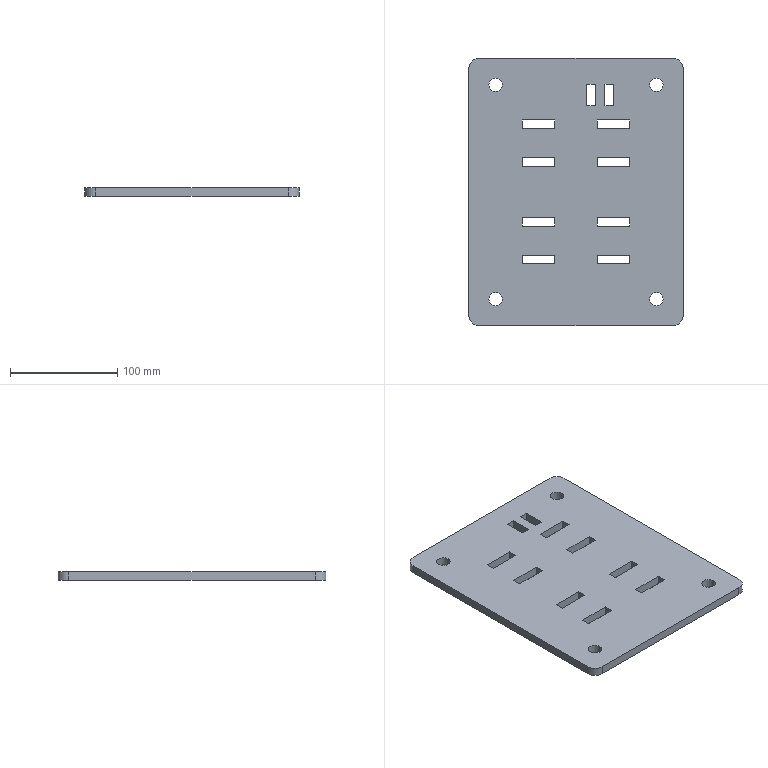Part | SolidWorks | features FlatPattern 1, SMBaseFlange 1, SheetMetal 1 | 1 solid | 58 faces | box 200 x 250 x 8 mm | volume 377466 mm3 | plane 46 | cylinder 12 | commonest cylinder face diameters 12.5 x8 20 x4